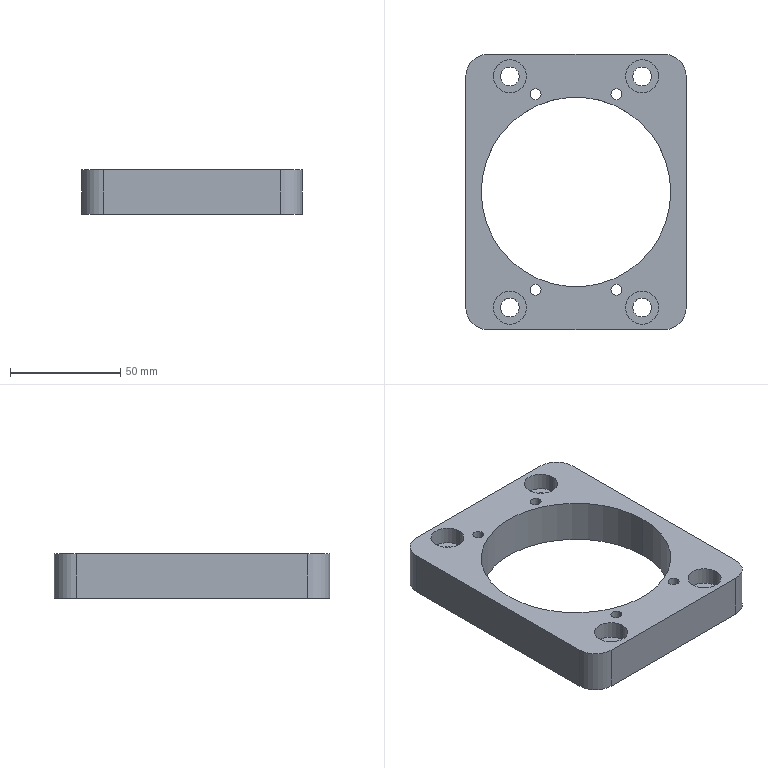Part | SolidWorks | features HoleWzd 2, Extrusion 1, Fillet 1, ICE 1, MirrorPattern 1 | 1 solid | 40 faces | box 100 x 125 x 20 mm | volume 122158 mm3 | cylinder 30 | plane 10 | commonest cylinder face diameters 5 x8 8.5 x8 15 x8 20 x4 86 x2
STEP:
#1=CARTESIAN_POINT('',(-20.869,-44.346,0.));
#2=VERTEX_POINT('',#1);
#3=CARTESIAN_POINT('',(-15.869,-44.346,0.));
#4=VERTEX_POINT('',#3);
#5=CARTESIAN_POINT('',(-18.369,-44.346,0.));
#6=DIRECTION('',(0.,0.,1.));
#7=DIRECTION('',(1.,0.,0.));
#8=AXIS2_PLACEMENT_3D('',#5,#6,#7);
#9=CIRCLE('',#8,2.5);
#10=EDGE_CURVE('',#2,#4,#9,.T.);
#11=ORIENTED_EDGE('',*,*,#10,.F.);
#12=CARTESIAN_POINT('',(-20.869,-44.346,20.));
#13=VERTEX_POINT('',#12);
#14=CARTESIAN_POINT('',(-20.869,-44.346,20.));
#15=DIRECTION('',(0.,0.,1.));
#16=VECTOR('',#15,1000.);
#17=LINE('',#14,#16);
#18=EDGE_CURVE('',#2,#13,#17,.T.);
#19=ORIENTED_EDGE('',*,*,#18,.T.);
#20=CARTESIAN_POINT('',(-15.869,-44.346,20.));
#21=VERTEX_POINT('',#20);
#22=CARTESIAN_POINT('',(-18.369,-44.346,20.));
#23=DIRECTION('',(0.,0.,1.));
#24=DIRECTION('',(1.,0.,0.));
#25=AXIS2_PLACEMENT_3D('',#22,#23,#24);
#26=CIRCLE('',#25,2.5);
#27=EDGE_CURVE('',#13,#21,#26,.T.);
#28=ORIENTED_EDGE('',*,*,#27,.T.);
#29=CARTESIAN_POINT('',(-15.869,-44.346,20.));
#30=DIRECTION('',(0.,0.,1.));
#31=VECTOR('',#30,1000.);
#32=LINE('',#29,#31);
#33=EDGE_CURVE('',#4,#21,#32,.T.);
#34=ORIENTED_EDGE('',*,*,#33,.F.);
#35=EDGE_LOOP('',(#11,#19,#28,#34));
#36=FACE_OUTER_BOUND('',#35,.T.);
#37=CARTESIAN_POINT('',(-18.369,-44.346,20.));
#38=DIRECTION('',(0.,0.,1.));
#39=DIRECTION('',(1.,0.,0.));
#40=AXIS2_PLACEMENT_3D('',#37,#38,#39);
#41=CYLINDRICAL_SURFACE('',#40,2.5);
#42=ADVANCED_FACE('',(#36),#41,.F.);
#43=CARTESIAN_POINT('',(15.869,-44.346,0.));
#44=VERTEX_POINT('',#43);
#45=CARTESIAN_POINT('',(20.869,-44.346,0.));
#46=VERTEX_POINT('',#45);
#47=CARTESIAN_POINT('',(18.369,-44.346,0.));
#48=DIRECTION('',(0.,0.,1.));
#49=DIRECTION('',(1.,0.,0.));
#50=AXIS2_PLACEMENT_3D('',#47,#48,#49);
#51=CIRCLE('',#50,2.5);
#52=EDGE_CURVE('',#44,#46,#51,.T.);
#53=ORIENTED_EDGE('',*,*,#52,.F.);
#54=CARTESIAN_POINT('',(15.869,-44.346,20.));
#55=VERTEX_POINT('',#54);
#56=CARTESIAN_POINT('',(15.869,-44.346,20.));
#57=DIRECTION('',(0.,0.,1.));
#58=VECTOR('',#57,1000.);
#59=LINE('',#56,#58);
#60=EDGE_CURVE('',#44,#55,#59,.T.);
#61=ORIENTED_EDGE('',*,*,#60,.T.);
#62=CARTESIAN_POINT('',(20.869,-44.346,20.));
#63=VERTEX_POINT('',#62);
#64=CARTESIAN_POINT('',(18.369,-44.346,20.));
#65=DIRECTION('',(0.,0.,1.));
#66=DIRECTION('',(1.,0.,0.));
#67=AXIS2_PLACEMENT_3D('',#64,#65,#66);
#68=CIRCLE('',#67,2.5);
#69=EDGE_CURVE('',#55,#63,#68,.T.);
#70=ORIENTED_EDGE('',*,*,#69,.T.);
#71=CARTESIAN_POINT('',(20.869,-44.346,20.));
#72=DIRECTION('',(0.,0.,1.));
#73=VECTOR('',#72,1000.);
#74=LINE('',#71,#73);
#75=EDGE_CURVE('',#46,#63,#74,.T.);
#76=ORIENTED_EDGE('',*,*,#75,.F.);
#77=EDGE_LOOP('',(#53,#61,#70,#76));
#78=FACE_OUTER_BOUND('',#77,.T.);
#79=CARTESIAN_POINT('',(18.369,-44.346,20.));
#80=DIRECTION('',(0.,0.,1.));
#81=DIRECTION('',(1.,0.,0.));
#82=AXIS2_PLACEMENT_3D('',#79,#80,#81);
#83=CYLINDRICAL_SURFACE('',#82,2.5);
#84=ADVANCED_FACE('',(#78),#83,.F.);
#85=CARTESIAN_POINT('',(-37.5,52.5,12.));
#86=VERTEX_POINT('',#85);
#87=CARTESIAN_POINT('',(-22.5,52.5,12.));
#88=VERTEX_POINT('',#87);
#89=CARTESIAN_POINT('',(-30.,52.5,12.));
#90=DIRECTION('',(0.,0.,1.));
#91=DIRECTION('',(1.,0.,0.));
#92=AXIS2_PLACEMENT_3D('',#89,#90,#91);
#93=CIRCLE('',#92,7.5);
#94=EDGE_CURVE('',#86,#88,#93,.T.);
#95=ORIENTED_EDGE('',*,*,#94,.F.);
#96=CARTESIAN_POINT('',(-37.5,52.5,20.));
#97=VERTEX_POINT('',#96);
#98=CARTESIAN_POINT('',(-37.5,52.5,20.));
#99=DIRECTION('',(0.,0.,1.));
#100=VECTOR('',#99,1000.);
#101=LINE('',#98,#100);
#102=EDGE_CURVE('',#86,#97,#101,.T.);
#103=ORIENTED_EDGE('',*,*,#102,.T.);
#104=CARTESIAN_POINT('',(-22.5,52.5,20.));
#105=VERTEX_POINT('',#104);
#106=CARTESIAN_POINT('',(-30.,52.5,20.));
#107=DIRECTION('',(0.,0.,1.));
#108=DIRECTION('',(1.,0.,0.));
#109=AXIS2_PLACEMENT_3D('',#106,#107,#108);
#110=CIRCLE('',#109,7.5);
#111=EDGE_CURVE('',#97,#105,#110,.T.);
#112=ORIENTED_EDGE('',*,*,#111,.T.);
#113=CARTESIAN_POINT('',(-22.5,52.5,20.));
#114=DIRECTION('',(0.,0.,1.));
#115=VECTOR('',#114,1000.);
#116=LINE('',#113,#115);
#117=EDGE_CURVE('',#88,#105,#116,.T.);
#118=ORIENTED_EDGE('',*,*,#117,.F.);
#119=EDGE_LOOP('',(#95,#103,#112,#118));
#120=FACE_OUTER_BOUND('',#119,.T.);
#121=CARTESIAN_POINT('',(-30.,52.5,20.));
#122=DIRECTION('',(0.,0.,1.));
#123=DIRECTION('',(1.,0.,0.));
#124=AXIS2_PLACEMENT_3D('',#121,#122,#123);
#125=CYLINDRICAL_SURFACE('',#124,7.5);
#126=ADVANCED_FACE('',(#120),#125,.F.);
#127=CARTESIAN_POINT('',(-34.25,52.5,0.));
#128=VERTEX_POINT('',#127);
#129=CARTESIAN_POINT('',(-25.75,52.5,0.));
#130=VERTEX_POINT('',#129);
#131=CARTESIAN_POINT('',(-30.,52.5,0.));
#132=DIRECTION('',(0.,0.,1.));
#133=DIRECTION('',(1.,0.,0.));
#134=AXIS2_PLACEMENT_3D('',#131,#132,#133);
#135=CIRCLE('',#134,4.25);
#136=EDGE_CURVE('',#128,#130,#135,.T.);
#137=ORIENTED_EDGE('',*,*,#136,.F.);
#138=CARTESIAN_POINT('',(-34.25,52.5,12.));
#139=VERTEX_POINT('',#138);
#140=CARTESIAN_POINT('',(-34.25,52.5,20.));
#141=DIRECTION('',(0.,0.,1.));
#142=VECTOR('',#141,1000.);
#143=LINE('',#140,#142);
#144=EDGE_CURVE('',#128,#139,#143,.T.);
#145=ORIENTED_EDGE('',*,*,#144,.T.);
#146=CARTESIAN_POINT('',(-25.75,52.5,12.));
#147=VERTEX_POINT('',#146);
#148=CARTESIAN_POINT('',(-30.,52.5,12.));
#149=DIRECTION('',(0.,0.,1.));
#150=DIRECTION('',(1.,0.,0.));
#151=AXIS2_PLACEMENT_3D('',#148,#149,#150);
#152=CIRCLE('',#151,4.25);
#153=EDGE_CURVE('',#139,#147,#152,.T.);
#154=ORIENTED_EDGE('',*,*,#153,.T.);
#155=CARTESIAN_POINT('',(-25.75,52.5,20.));
#156=DIRECTION('',(0.,0.,1.));
#157=VECTOR('',#156,1000.);
#158=LINE('',#155,#157);
#159=EDGE_CURVE('',#130,#147,#158,.T.);
#160=ORIENTED_EDGE('',*,*,#159,.F.);
#161=EDGE_LOOP('',(#137,#145,#154,#160));
#162=FACE_OUTER_BOUND('',#161,.T.);
#163=CARTESIAN_POINT('',(-30.,52.5,20.));
#164=DIRECTION('',(0.,0.,1.));
#165=DIRECTION('',(1.,0.,0.));
#166=AXIS2_PLACEMENT_3D('',#163,#164,#165);
#167=CYLINDRICAL_SURFACE('',#166,4.25);
#168=ADVANCED_FACE('',(#162),#167,.F.);
#169=CARTESIAN_POINT('',(22.5,52.5,12.));
#170=VERTEX_POINT('',#169);
#171=CARTESIAN_POINT('',(37.5,52.5,12.));
#172=VERTEX_POINT('',#171);
#173=CARTESIAN_POINT('',(30.,52.5,12.));
#174=DIRECTION('',(0.,0.,1.));
#175=DIRECTION('',(1.,0.,0.));
#176=AXIS2_PLACEMENT_3D('',#173,#174,#175);
#177=CIRCLE('',#176,7.5);
#178=EDGE_CURVE('',#170,#172,#177,.T.);
#179=ORIENTED_EDGE('',*,*,#178,.F.);
#180=CARTESIAN_POINT('',(22.5,52.5,20.));
#181=VERTEX_POINT('',#180);
#182=CARTESIAN_POINT('',(22.5,52.5,20.));
#183=DIRECTION('',(0.,0.,1.));
#184=VECTOR('',#183,1000.);
#185=LINE('',#182,#184);
#186=EDGE_CURVE('',#170,#181,#185,.T.);
#187=ORIENTED_EDGE('',*,*,#186,.T.);
#188=CARTESIAN_POINT('',(37.5,52.5,20.));
#189=VERTEX_POINT('',#188);
#190=CARTESIAN_POINT('',(30.,52.5,20.));
#191=DIRECTION('',(0.,0.,1.));
#192=DIRECTION('',(1.,0.,0.));
#193=AXIS2_PLACEMENT_3D('',#190,#191,#192);
#194=CIRCLE('',#193,7.5);
#195=EDGE_CURVE('',#181,#189,#194,.T.);
#196=ORIENTED_EDGE('',*,*,#195,.T.);
#197=CARTESIAN_POINT('',(37.5,52.5,20.));
#198=DIRECTION('',(0.,0.,1.));
#199=VECTOR('',#198,1000.);
#200=LINE('',#197,#199);
#201=EDGE_CURVE('',#172,#189,#200,.T.);
#202=ORIENTED_EDGE('',*,*,#201,.F.);
#203=EDGE_LOOP('',(#179,#187,#196,#202));
#204=FACE_OUTER_BOUND('',#203,.T.);
#205=CARTESIAN_POINT('',(30.,52.5,20.));
#206=DIRECTION('',(0.,0.,1.));
#207=DIRECTION('',(1.,0.,0.));
#208=AXIS2_PLACEMENT_3D('',#205,#206,#207);
#209=CYLINDRICAL_SURFACE('',#208,7.5);
#210=ADVANCED_FACE('',(#204),#209,.F.);
#211=CARTESIAN_POINT('',(25.75,52.5,0.));
#212=VERTEX_POINT('',#211);
#213=CARTESIAN_POINT('',(34.25,52.5,0.));
#214=VERTEX_POINT('',#213);
#215=CARTESIAN_POINT('',(30.,52.5,0.));
#216=DIRECTION('',(0.,0.,1.));
#217=DIRECTION('',(1.,0.,0.));
#218=AXIS2_PLACEMENT_3D('',#215,#216,#217);
#219=CIRCLE('',#218,4.25);
#220=EDGE_CURVE('',#212,#214,#219,.T.);
#221=ORIENTED_EDGE('',*,*,#220,.F.);
#222=CARTESIAN_POINT('',(25.75,52.5,12.));
#223=VERTEX_POINT('',#222);
#224=CARTESIAN_POINT('',(25.75,52.5,20.));
#225=DIRECTION('',(0.,0.,1.));
#226=VECTOR('',#225,1000.);
#227=LINE('',#224,#226);
#228=EDGE_CURVE('',#212,#223,#227,.T.);
#229=ORIENTED_EDGE('',*,*,#228,.T.);
#230=CARTESIAN_POINT('',(34.25,52.5,12.));
#231=VERTEX_POINT('',#230);
#232=CARTESIAN_POINT('',(30.,52.5,12.));
#233=DIRECTION('',(0.,0.,1.));
#234=DIRECTION('',(1.,0.,0.));
#235=AXIS2_PLACEMENT_3D('',#232,#233,#234);
#236=CIRCLE('',#235,4.25);
#237=EDGE_CURVE('',#223,#231,#236,.T.);
#238=ORIENTED_EDGE('',*,*,#237,.T.);
#239=CARTESIAN_POINT('',(34.25,52.5,20.));
#240=DIRECTION('',(0.,0.,1.));
#241=VECTOR('',#240,1000.);
#242=LINE('',#239,#241);
#243=EDGE_CURVE('',#214,#231,#242,.T.);
#244=ORIENTED_EDGE('',*,*,#243,.F.);
#245=EDGE_LOOP('',(#221,#229,#238,#244));
#246=FACE_OUTER_BOUND('',#245,.T.);
#247=CARTESIAN_POINT('',(30.,52.5,20.));
#248=DIRECTION('',(0.,0.,1.));
#249=DIRECTION('',(1.,0.,0.));
#250=AXIS2_PLACEMENT_3D('',#247,#248,#249);
#251=CYLINDRICAL_SURFACE('',#250,4.25);
#252=ADVANCED_FACE('',(#246),#251,.F.);
#253=CARTESIAN_POINT('',(-20.869,44.346,0.));
#254=VERTEX_POINT('',#253);
#255=CARTESIAN_POINT('',(-15.869,44.346,0.));
#256=VERTEX_POINT('',#255);
#257=CARTESIAN_POINT('',(-18.369,44.346,0.));
#258=DIRECTION('',(0.,0.,1.));
#259=DIRECTION('',(1.,0.,0.));
#260=AXIS2_PLACEMENT_3D('',#257,#258,#259);
#261=CIRCLE('',#260,2.5);
#262=EDGE_CURVE('',#254,#256,#261,.T.);
#263=ORIENTED_EDGE('',*,*,#262,.F.);
#264=CARTESIAN_POINT('',(-20.869,44.346,20.));
#265=VERTEX_POINT('',#264);
#266=CARTESIAN_POINT('',(-20.869,44.346,20.));
#267=DIRECTION('',(0.,0.,1.));
#268=VECTOR('',#267,1000.);
#269=LINE('',#266,#268);
#270=EDGE_CURVE('',#254,#265,#269,.T.);
#271=ORIENTED_EDGE('',*,*,#270,.T.);
#272=CARTESIAN_POINT('',(-15.869,44.346,20.));
#273=VERTEX_POINT('',#272);
#274=CARTESIAN_POINT('',(-18.369,44.346,20.));
#275=DIRECTION('',(0.,0.,1.));
#276=DIRECTION('',(1.,0.,0.));
#277=AXIS2_PLACEMENT_3D('',#274,#275,#276);
#278=CIRCLE('',#277,2.5);
#279=EDGE_CURVE('',#265,#273,#278,.T.);
#280=ORIENTED_EDGE('',*,*,#279,.T.);
#281=CARTESIAN_POINT('',(-15.869,44.346,20.));
#282=DIRECTION('',(0.,0.,1.));
#283=VECTOR('',#282,1000.);
#284=LINE('',#281,#283);
#285=EDGE_CURVE('',#256,#273,#284,.T.);
#286=ORIENTED_EDGE('',*,*,#285,.F.);
#287=EDGE_LOOP('',(#263,#271,#280,#286));
#288=FACE_OUTER_BOUND('',#287,.T.);
#289=CARTESIAN_POINT('',(-18.369,44.346,20.));
#290=DIRECTION('',(0.,0.,1.));
#291=DIRECTION('',(1.,0.,0.));
#292=AXIS2_PLACEMENT_3D('',#289,#290,#291);
#293=CYLINDRICAL_SURFACE('',#292,2.5);
#294=ADVANCED_FACE('',(#288),#293,.F.);
#295=CARTESIAN_POINT('',(15.869,44.346,0.));
#296=VERTEX_POINT('',#295);
#297=CARTESIAN_POINT('',(20.869,44.346,0.));
#298=VERTEX_POINT('',#297);
#299=CARTESIAN_POINT('',(18.369,44.346,0.));
#300=DIRECTION('',(0.,0.,1.));
#301=DIRECTION('',(1.,0.,0.));
#302=AXIS2_PLACEMENT_3D('',#299,#300,#301);
#303=CIRCLE('',#302,2.5);
#304=EDGE_CURVE('',#296,#298,#303,.T.);
#305=ORIENTED_EDGE('',*,*,#304,.F.);
#306=CARTESIAN_POINT('',(15.869,44.346,20.));
#307=VERTEX_POINT('',#306);
#308=CARTESIAN_POINT('',(15.869,44.346,20.));
#309=DIRECTION('',(0.,0.,1.));
#310=VECTOR('',#309,1000.);
#311=LINE('',#308,#310);
#312=EDGE_CURVE('',#296,#307,#311,.T.);
#313=ORIENTED_EDGE('',*,*,#312,.T.);
#314=CARTESIAN_POINT('',(20.869,44.346,20.));
#315=VERTEX_POINT('',#314);
#316=CARTESIAN_POINT('',(18.369,44.346,20.));
#317=DIRECTION('',(0.,0.,1.));
#318=DIRECTION('',(1.,0.,0.));
#319=AXIS2_PLACEMENT_3D('',#316,#317,#318);
#320=CIRCLE('',#319,2.5);
#321=EDGE_CURVE('',#307,#315,#320,.T.);
#322=ORIENTED_EDGE('',*,*,#321,.T.);
#323=CARTESIAN_POINT('',(20.869,44.346,20.));
#324=DIRECTION('',(0.,0.,1.));
#325=VECTOR('',#324,1000.);
#326=LINE('',#323,#325);
#327=EDGE_CURVE('',#298,#315,#326,.T.);
#328=ORIENTED_EDGE('',*,*,#327,.F.);
#329=EDGE_LOOP('',(#305,#313,#322,#328));
#330=FACE_OUTER_BOUND('',#329,.T.);
#331=CARTESIAN_POINT('',(18.369,44.346,20.));
#332=DIRECTION('',(0.,0.,1.));
#333=DIRECTION('',(1.,0.,0.));
#334=AXIS2_PLACEMENT_3D('',#331,#332,#333);
#335=CYLINDRICAL_SURFACE('',#334,2.5);
#336=ADVANCED_FACE('',(#330),#335,.F.);
#337=CARTESIAN_POINT('',(-43.,0.,0.));
#338=VERTEX_POINT('',#337);
#339=CARTESIAN_POINT('',(43.,0.,0.));
#340=VERTEX_POINT('',#339);
#341=CARTESIAN_POINT('',(0.,0.,0.));
#342=DIRECTION('',(0.,0.,1.));
#343=DIRECTION('',(1.,0.,0.));
#344=AXIS2_PLACEMENT_3D('',#341,#342,#343);
#345=CIRCLE('',#344,43.);
#346=EDGE_CURVE('',#338,#340,#345,.T.);
#347=ORIENTED_EDGE('',*,*,#346,.F.);
#348=CARTESIAN_POINT('',(-43.,0.,20.));
#349=VERTEX_POINT('',#348);
#350=CARTESIAN_POINT('',(-43.,0.,0.));
#351=DIRECTION('',(0.,0.,1.));
#352=VECTOR('',#351,1000.);
#353=LINE('',#350,#352);
#354=EDGE_CURVE('',#338,#349,#353,.T.);
#355=ORIENTED_EDGE('',*,*,#354,.T.);
#356=CARTESIAN_POINT('',(43.,0.,20.));
#357=VERTEX_POINT('',#356);
#358=CARTESIAN_POINT('',(0.,0.,20.));
#359=DIRECTION('',(0.,0.,1.));
#360=DIRECTION('',(1.,0.,0.));
#361=AXIS2_PLACEMENT_3D('',#358,#359,#360);
#362=CIRCLE('',#361,43.);
#363=EDGE_CURVE('',#349,#357,#362,.T.);
#364=ORIENTED_EDGE('',*,*,#363,.T.);
#365=CARTESIAN_POINT('',(43.,0.,0.));
#366=DIRECTION('',(0.,0.,1.));
#367=VECTOR('',#366,1000.);
#368=LINE('',#365,#367);
#369=EDGE_CURVE('',#340,#357,#368,.T.);
#370=ORIENTED_EDGE('',*,*,#369,.F.);
#371=EDGE_LOOP('',(#347,#355,#364,#370));
#372=FACE_OUTER_BOUND('',#371,.T.);
#373=CARTESIAN_POINT('',(0.,0.,0.));
#374=DIRECTION('',(0.,0.,1.));
#375=DIRECTION('',(1.,0.,0.));
#376=AXIS2_PLACEMENT_3D('',#373,#374,#375);
#377=CYLINDRICAL_SURFACE('',#376,43.);
#378=ADVANCED_FACE('',(#372),#377,.F.);
#379=CARTESIAN_POINT('',(-37.5,-52.5,12.));
#380=VERTEX_POINT('',#379);
#381=CARTESIAN_POINT('',(-22.5,-52.5,12.));
#382=VERTEX_POINT('',#381);
#383=CARTESIAN_POINT('',(-30.,-52.5,12.));
#384=DIRECTION('',(0.,0.,1.));
#385=DIRECTION('',(1.,0.,0.));
#386=AXIS2_PLACEMENT_3D('',#383,#384,#385);
#387=CIRCLE('',#386,7.5);
#388=EDGE_CURVE('',#380,#382,#387,.T.);
#389=ORIENTED_EDGE('',*,*,#388,.F.);
#390=CARTESIAN_POINT('',(-37.5,-52.5,20.));
#391=VERTEX_POINT('',#390);
#392=CARTESIAN_POINT('',(-37.5,-52.5,20.));
#393=DIRECTION('',(0.,0.,1.));
#394=VECTOR('',#393,1000.);
#395=LINE('',#392,#394);
#396=EDGE_CURVE('',#380,#391,#395,.T.);
#397=ORIENTED_EDGE('',*,*,#396,.T.);
#398=CARTESIAN_POINT('',(-22.5,-52.5,20.));
#399=VERTEX_POINT('',#398);
#400=CARTESIAN_POINT('',(-30.,-52.5,20.));
#401=DIRECTION('',(0.,0.,1.));
#402=DIRECTION('',(1.,0.,0.));
#403=AXIS2_PLACEMENT_3D('',#400,#401,#402);
#404=CIRCLE('',#403,7.5);
#405=EDGE_CURVE('',#391,#399,#404,.T.);
#406=ORIENTED_EDGE('',*,*,#405,.T.);
#407=CARTESIAN_POINT('',(-22.5,-52.5,20.));
#408=DIRECTION('',(0.,0.,1.));
#409=VECTOR('',#408,1000.);
#410=LINE('',#407,#409);
#411=EDGE_CURVE('',#382,#399,#410,.T.);
#412=ORIENTED_EDGE('',*,*,#411,.F.);
#413=EDGE_LOOP('',(#389,#397,#406,#412));
#414=FACE_OUTER_BOUND('',#413,.T.);
#415=CARTESIAN_POINT('',(-30.,-52.5,20.));
#416=DIRECTION('',(0.,0.,1.));
#417=DIRECTION('',(1.,0.,0.));
#418=AXIS2_PLACEMENT_3D('',#415,#416,#417);
#419=CYLINDRICAL_SURFACE('',#418,7.5);
#420=ADVANCED_FACE('',(#414),#419,.F.);
#421=CARTESIAN_POINT('',(-34.25,-52.5,0.));
#422=VERTEX_POINT('',#421);
#423=CARTESIAN_POINT('',(-25.75,-52.5,0.));
#424=VERTEX_POINT('',#423);
#425=CARTESIAN_POINT('',(-30.,-52.5,0.));
#426=DIRECTION('',(0.,0.,1.));
#427=DIRECTION('',(1.,0.,0.));
#428=AXIS2_PLACEMENT_3D('',#425,#426,#427);
#429=CIRCLE('',#428,4.25);
#430=EDGE_CURVE('',#422,#424,#429,.T.);
#431=ORIENTED_EDGE('',*,*,#430,.F.);
#432=CARTESIAN_POINT('',(-34.25,-52.5,12.));
#433=VERTEX_POINT('',#432);
#434=CARTESIAN_POINT('',(-34.25,-52.5,20.));
#435=DIRECTION('',(0.,0.,1.));
#436=VECTOR('',#435,1000.);
#437=LINE('',#434,#436);
#438=EDGE_CURVE('',#422,#433,#437,.T.);
#439=ORIENTED_EDGE('',*,*,#438,.T.);
#440=CARTESIAN_POINT('',(-25.75,-52.5,12.));
#441=VERTEX_POINT('',#440);
#442=CARTESIAN_POINT('',(-30.,-52.5,12.));
#443=DIRECTION('',(0.,0.,1.));
#444=DIRECTION('',(1.,0.,0.));
#445=AXIS2_PLACEMENT_3D('',#442,#443,#444);
#446=CIRCLE('',#445,4.25);
#447=EDGE_CURVE('',#433,#441,#446,.T.);
#448=ORIENTED_EDGE('',*,*,#447,.T.);
#449=CARTESIAN_POINT('',(-25.75,-52.5,20.));
#450=DIRECTION('',(0.,0.,1.));
#451=VECTOR('',#450,1000.);
#452=LINE('',#449,#451);
#453=EDGE_CURVE('',#424,#441,#452,.T.);
#454=ORIENTED_EDGE('',*,*,#453,.F.);
#455=EDGE_LOOP('',(#431,#439,#448,#454));
#456=FACE_OUTER_BOUND('',#455,.T.);
#457=CARTESIAN_POINT('',(-30.,-52.5,20.));
#458=DIRECTION('',(0.,0.,1.));
#459=DIRECTION('',(1.,0.,0.));
#460=AXIS2_PLACEMENT_3D('',#457,#458,#459);
#461=CYLINDRICAL_SURFACE('',#460,4.25);
#462=ADVANCED_FACE('',(#456),#461,.F.);
#463=CARTESIAN_POINT('',(22.5,-52.5,12.));
#464=VERTEX_POINT('',#463);
#465=CARTESIAN_POINT('',(37.5,-52.5,12.));
#466=VERTEX_POINT('',#465);
#467=CARTESIAN_POINT('',(30.,-52.5,12.));
#468=DIRECTION('',(0.,0.,1.));
#469=DIRECTION('',(1.,0.,0.));
#470=AXIS2_PLACEMENT_3D('',#467,#468,#469);
#471=CIRCLE('',#470,7.5);
#472=EDGE_CURVE('',#464,#466,#471,.T.);
#473=ORIENTED_EDGE('',*,*,#472,.F.);
#474=CARTESIAN_POINT('',(22.5,-52.5,20.));
#475=VERTEX_POINT('',#474);
#476=CARTESIAN_POINT('',(22.5,-52.5,20.));
#477=DIRECTION('',(0.,0.,1.));
#478=VECTOR('',#477,1000.);
#479=LINE('',#476,#478);
#480=EDGE_CURVE('',#464,#475,#479,.T.);
#481=ORIENTED_EDGE('',*,*,#480,.T.);
#482=CARTESIAN_POINT('',(37.5,-52.5,20.));
#483=VERTEX_POINT('',#482);
#484=CARTESIAN_POINT('',(30.,-52.5,20.));
#485=DIRECTION('',(0.,0.,1.));
#486=DIRECTION('',(1.,0.,0.));
#487=AXIS2_PLACEMENT_3D('',#484,#485,#486);
#488=CIRCLE('',#487,7.5);
#489=EDGE_CURVE('',#475,#483,#488,.T.);
#490=ORIENTED_EDGE('',*,*,#489,.T.);
#491=CARTESIAN_POINT('',(37.5,-52.5,20.));
#492=DIRECTION('',(0.,0.,1.));
#493=VECTOR('',#492,1000.);
#494=LINE('',#491,#493);
#495=EDGE_CURVE('',#466,#483,#494,.T.);
#496=ORIENTED_EDGE('',*,*,#495,.F.);
#497=EDGE_LOOP('',(#473,#481,#490,#496));
#498=FACE_OUTER_BOUND('',#497,.T.);
#499=CARTESIAN_POINT('',(30.,-52.5,20.));
#500=DIRECTION('',(0.,0.,1.));
#501=DIRECTION('',(1.,0.,0.));
#502=AXIS2_PLACEMENT_3D('',#499,#500,#501);
#503=CYLINDRICAL_SURFACE('',#502,7.5);
#504=ADVANCED_FACE('',(#498),#503,.F.);
#505=CARTESIAN_POINT('',(25.75,-52.5,0.));
#506=VERTEX_POINT('',#505);
#507=CARTESIAN_POINT('',(34.25,-52.5,0.));
#508=VERTEX_POINT('',#507);
#509=CARTESIAN_POINT('',(30.,-52.5,0.));
#510=DIRECTION('',(0.,0.,1.));
#511=DIRECTION('',(1.,0.,0.));
#512=AXIS2_PLACEMENT_3D('',#509,#510,#511);
#513=CIRCLE('',#512,4.25);
#514=EDGE_CURVE('',#506,#508,#513,.T.);
#515=ORIENTED_EDGE('',*,*,#514,.F.);
#516=CARTESIAN_POINT('',(25.75,-52.5,12.));
#517=VERTEX_POINT('',#516);
#518=CARTESIAN_POINT('',(25.75,-52.5,20.));
#519=DIRECTION('',(0.,0.,1.));
#520=VECTOR('',#519,1000.);
#521=LINE('',#518,#520);
#522=EDGE_CURVE('',#506,#517,#521,.T.);
#523=ORIENTED_EDGE('',*,*,#522,.T.);
#524=CARTESIAN_POINT('',(34.25,-52.5,12.));
#525=VERTEX_POINT('',#524);
#526=CARTESIAN_POINT('',(30.,-52.5,12.));
#527=DIRECTION('',(0.,0.,1.));
#528=DIRECTION('',(1.,0.,0.));
#529=AXIS2_PLACEMENT_3D('',#526,#527,#528);
#530=CIRCLE('',#529,4.25);
#531=EDGE_CURVE('',#517,#525,#530,.T.);
#532=ORIENTED_EDGE('',*,*,#531,.T.);
#533=CARTESIAN_POINT('',(34.25,-52.5,20.));
#534=DIRECTION('',(0.,0.,1.));
#535=VECTOR('',#534,1000.);
#536=LINE('',#533,#535);
#537=EDGE_CURVE('',#508,#525,#536,.T.);
#538=ORIENTED_EDGE('',*,*,#537,.F.);
#539=EDGE_LOOP('',(#515,#523,#532,#538));
#540=FACE_OUTER_BOUND('',#539,.T.);
#541=CARTESIAN_POINT('',(30.,-52.5,20.));
#542=DIRECTION('',(0.,0.,1.));
#543=DIRECTION('',(1.,0.,0.));
#544=AXIS2_PLACEMENT_3D('',#541,#542,#543);
#545=CYLINDRICAL_SURFACE('',#544,4.25);
#546=ADVANCED_FACE('',(#540),#545,.F.);
#547=CARTESIAN_POINT('',(-50.,52.5,0.));
#548=VERTEX_POINT('',#547);
#549=CARTESIAN_POINT('',(-50.,-52.5,0.));
#550=VERTEX_POINT('',#549);
#551=CARTESIAN_POINT('',(-50.,62.5,0.));
#552=DIRECTION('',(0.,-1.,0.));
#553=VECTOR('',#552,1000.);
#554=LINE('',#551,#553);
#555=EDGE_CURVE('',#548,#550,#554,.T.);
#556=ORIENTED_EDGE('',*,*,#555,.T.);
#557=CARTESIAN_POINT('',(-50.,-52.5,20.));
#558=VERTEX_POINT('',#557);
#559=CARTESIAN_POINT('',(-50.,-52.5,20.));
#560=DIRECTION('',(0.,0.,1.));
#561=VECTOR('',#560,1000.);
#562=LINE('',#559,#561);
#563=EDGE_CURVE('',#550,#558,#562,.T.);
#564=ORIENTED_EDGE('',*,*,#563,.T.);
#565=CARTESIAN_POINT('',(-50.,52.5,20.));
#566=VERTEX_POINT('',#565);
#567=CARTESIAN_POINT('',(-50.,62.5,20.));
#568=DIRECTION('',(0.,-1.,0.));
#569=VECTOR('',#568,1000.);
#570=LINE('',#567,#569);
#571=EDGE_CURVE('',#566,#558,#570,.T.);
#572=ORIENTED_EDGE('',*,*,#571,.F.);
#573=CARTESIAN_POINT('',(-50.,52.5,0.));
#574=DIRECTION('',(0.,0.,-1.));
#575=VECTOR('',#574,1000.);
#576=LINE('',#573,#575);
#577=EDGE_CURVE('',#566,#548,#576,.T.);
#578=ORIENTED_EDGE('',*,*,#577,.T.);
#579=EDGE_LOOP('',(#556,#564,#572,#578));
#580=FACE_OUTER_BOUND('',#579,.T.);
#581=CARTESIAN_POINT('',(-50.,62.5,20.));
#582=DIRECTION('',(1.,0.,0.));
#583=DIRECTION('',(0.,1.,0.));
#584=AXIS2_PLACEMENT_3D('',#581,#582,#583);
#585=PLANE('',#584);
#586=ADVANCED_FACE('',(#580),#585,.F.);
#587=CARTESIAN_POINT('',(-40.,-62.5,0.));
#588=VERTEX_POINT('',#587);
#589=CARTESIAN_POINT('',(40.,-62.5,0.));
#590=VERTEX_POINT('',#589);
#591=CARTESIAN_POINT('',(-50.,-62.5,0.));
#592=DIRECTION('',(1.,0.,0.));
#593=VECTOR('',#592,1000.);
#594=LINE('',#591,#593);
#595=EDGE_CURVE('',#588,#590,#594,.T.);
#596=ORIENTED_EDGE('',*,*,#595,.T.);
#597=CARTESIAN_POINT('',(40.,-62.5,20.));
#598=VERTEX_POINT('',#597);
#599=CARTESIAN_POINT('',(40.,-62.5,20.));
#600=DIRECTION('',(0.,0.,1.));
#601=VECTOR('',#600,1000.);
#602=LINE('',#599,#601);
#603=EDGE_CURVE('',#590,#598,#602,.T.);
#604=ORIENTED_EDGE('',*,*,#603,.T.);
#605=CARTESIAN_POINT('',(-40.,-62.5,20.));
#606=VERTEX_POINT('',#605);
#607=CARTESIAN_POINT('',(-50.,-62.5,20.));
#608=DIRECTION('',(1.,0.,0.));
#609=VECTOR('',#608,1000.);
#610=LINE('',#607,#609);
#611=EDGE_CURVE('',#606,#598,#610,.T.);
#612=ORIENTED_EDGE('',*,*,#611,.F.);
#613=CARTESIAN_POINT('',(-40.,-62.5,20.));
#614=DIRECTION('',(0.,0.,-1.));
#615=VECTOR('',#614,1000.);
#616=LINE('',#613,#615);
#617=EDGE_CURVE('',#606,#588,#616,.T.);
#618=ORIENTED_EDGE('',*,*,#617,.T.);
#619=EDGE_LOOP('',(#596,#604,#612,#618));
#620=FACE_OUTER_BOUND('',#619,.T.);
#621=CARTESIAN_POINT('',(-50.,-62.5,20.));
#622=DIRECTION('',(0.,1.,0.));
#623=DIRECTION('',(0.,0.,1.));
#624=AXIS2_PLACEMENT_3D('',#621,#622,#623);
#625=PLANE('',#624);
#626=ADVANCED_FACE('',(#620),#625,.F.);
#627=CARTESIAN_POINT('',(50.,52.5,0.));
#628=VERTEX_POINT('',#627);
#629=CARTESIAN_POINT('',(50.,-52.5,0.));
#630=VERTEX_POINT('',#629);
#631=CARTESIAN_POINT('',(50.,62.5,0.));
#632=DIRECTION('',(0.,-1.,0.));
#633=VECTOR('',#632,1000.);
#634=LINE('',#631,#633);
#635=EDGE_CURVE('',#628,#630,#634,.T.);
#636=ORIENTED_EDGE('',*,*,#635,.F.);
#637=CARTESIAN_POINT('',(50.,52.5,20.));
#638=VERTEX_POINT('',#637);
#639=CARTESIAN_POINT('',(50.,52.5,20.));
#640=DIRECTION('',(0.,0.,1.));
#641=VECTOR('',#640,1000.);
#642=LINE('',#639,#641);
#643=EDGE_CURVE('',#628,#638,#642,.T.);
#644=ORIENTED_EDGE('',*,*,#643,.T.);
#645=CARTESIAN_POINT('',(50.,-52.5,20.));
#646=VERTEX_POINT('',#645);
#647=CARTESIAN_POINT('',(50.,62.5,20.));
#648=DIRECTION('',(0.,-1.,0.));
#649=VECTOR('',#648,1000.);
#650=LINE('',#647,#649);
#651=EDGE_CURVE('',#638,#646,#650,.T.);
#652=ORIENTED_EDGE('',*,*,#651,.T.);
#653=CARTESIAN_POINT('',(50.,-52.5,0.));
#654=DIRECTION('',(0.,0.,-1.));
#655=VECTOR('',#654,1000.);
#656=LINE('',#653,#655);
#657=EDGE_CURVE('',#646,#630,#656,.T.);
#658=ORIENTED_EDGE('',*,*,#657,.T.);
#659=EDGE_LOOP('',(#636,#644,#652,#658));
#660=FACE_OUTER_BOUND('',#659,.T.);
#661=CARTESIAN_POINT('',(50.,62.5,20.));
#662=DIRECTION('',(1.,0.,0.));
#663=DIRECTION('',(0.,1.,0.));
#664=AXIS2_PLACEMENT_3D('',#661,#662,#663);
#665=PLANE('',#664);
#666=ADVANCED_FACE('',(#660),#665,.T.);
#667=CARTESIAN_POINT('',(-40.,62.5,20.));
#668=VERTEX_POINT('',#667);
#669=CARTESIAN_POINT('',(40.,62.5,20.));
#670=VERTEX_POINT('',#669);
#671=CARTESIAN_POINT('',(-50.,62.5,20.));
#672=DIRECTION('',(1.,0.,0.));
#673=VECTOR('',#672,1000.);
#674=LINE('',#671,#673);
#675=EDGE_CURVE('',#668,#670,#674,.T.);
#676=ORIENTED_EDGE('',*,*,#675,.T.);
#677=CARTESIAN_POINT('',(40.,62.5,0.));
#678=VERTEX_POINT('',#677);
#679=CARTESIAN_POINT('',(40.,62.5,20.));
#680=DIRECTION('',(0.,0.,-1.));
#681=VECTOR('',#680,1000.);
#682=LINE('',#679,#681);
#683=EDGE_CURVE('',#670,#678,#682,.T.);
#684=ORIENTED_EDGE('',*,*,#683,.T.);
#685=CARTESIAN_POINT('',(-40.,62.5,0.));
#686=VERTEX_POINT('',#685);
#687=CARTESIAN_POINT('',(-50.,62.5,0.));
#688=DIRECTION('',(1.,0.,0.));
#689=VECTOR('',#688,1000.);
#690=LINE('',#687,#689);
#691=EDGE_CURVE('',#686,#678,#690,.T.);
#692=ORIENTED_EDGE('',*,*,#691,.F.);
#693=CARTESIAN_POINT('',(-40.,62.5,20.));
#694=DIRECTION('',(0.,0.,1.));
#695=VECTOR('',#694,1000.);
#696=LINE('',#693,#695);
#697=EDGE_CURVE('',#686,#668,#696,.T.);
#698=ORIENTED_EDGE('',*,*,#697,.T.);
#699=EDGE_LOOP('',(#676,#684,#692,#698));
#700=FACE_OUTER_BOUND('',#699,.T.);
#701=CARTESIAN_POINT('',(-50.,62.5,20.));
#702=DIRECTION('',(0.,1.,0.));
#703=DIRECTION('',(0.,0.,1.));
#704=AXIS2_PLACEMENT_3D('',#701,#702,#703);
#705=PLANE('',#704);
#706=ADVANCED_FACE('',(#700),#705,.T.);
#707=CARTESIAN_POINT('',(-18.369,-44.346,20.));
#708=DIRECTION('',(0.,0.,1.));
#709=DIRECTION('',(1.,0.,0.));
#710=AXIS2_PLACEMENT_3D('',#707,#708,#709);
#711=CIRCLE('',#710,2.5);
#712=EDGE_CURVE('',#21,#13,#711,.T.);
#713=ORIENTED_EDGE('',*,*,#712,.F.);
#714=ORIENTED_EDGE('',*,*,#27,.F.);
#715=EDGE_LOOP('',(#713,#714));
#716=FACE_BOUND('',#715,.T.);
#717=CARTESIAN_POINT('',(18.369,-44.346,20.));
#718=DIRECTION('',(0.,0.,1.));
#719=DIRECTION('',(1.,0.,0.));
#720=AXIS2_PLACEMENT_3D('',#717,#718,#719);
#721=CIRCLE('',#720,2.5);
#722=EDGE_CURVE('',#63,#55,#721,.T.);
#723=ORIENTED_EDGE('',*,*,#722,.F.);
#724=ORIENTED_EDGE('',*,*,#69,.F.);
#725=EDGE_LOOP('',(#723,#724));
#726=FACE_BOUND('',#725,.T.);
#727=CARTESIAN_POINT('',(-30.,52.5,20.));
#728=DIRECTION('',(0.,0.,1.));
#729=DIRECTION('',(1.,0.,0.));
#730=AXIS2_PLACEMENT_3D('',#727,#728,#729);
#731=CIRCLE('',#730,7.5);
#732=EDGE_CURVE('',#105,#97,#731,.T.);
#733=ORIENTED_EDGE('',*,*,#732,.F.);
#734=ORIENTED_EDGE('',*,*,#111,.F.);
#735=EDGE_LOOP('',(#733,#734));
#736=FACE_BOUND('',#735,.T.);
#737=CARTESIAN_POINT('',(30.,52.5,20.));
#738=DIRECTION('',(0.,0.,1.));
#739=DIRECTION('',(1.,0.,0.));
#740=AXIS2_PLACEMENT_3D('',#737,#738,#739);
#741=CIRCLE('',#740,7.5);
#742=EDGE_CURVE('',#189,#181,#741,.T.);
#743=ORIENTED_EDGE('',*,*,#742,.F.);
#744=ORIENTED_EDGE('',*,*,#195,.F.);
#745=EDGE_LOOP('',(#743,#744));
#746=FACE_BOUND('',#745,.T.);
#747=CARTESIAN_POINT('',(-18.369,44.346,20.));
#748=DIRECTION('',(0.,0.,1.));
#749=DIRECTION('',(1.,0.,0.));
#750=AXIS2_PLACEMENT_3D('',#747,#748,#749);
#751=CIRCLE('',#750,2.5);
#752=EDGE_CURVE('',#273,#265,#751,.T.);
#753=ORIENTED_EDGE('',*,*,#752,.F.);
#754=ORIENTED_EDGE('',*,*,#279,.F.);
#755=EDGE_LOOP('',(#753,#754));
#756=FACE_BOUND('',#755,.T.);
#757=CARTESIAN_POINT('',(18.369,44.346,20.));
#758=DIRECTION('',(0.,0.,1.));
#759=DIRECTION('',(1.,0.,0.));
#760=AXIS2_PLACEMENT_3D('',#757,#758,#759);
#761=CIRCLE('',#760,2.5);
#762=EDGE_CURVE('',#315,#307,#761,.T.);
#763=ORIENTED_EDGE('',*,*,#762,.F.);
#764=ORIENTED_EDGE('',*,*,#321,.F.);
#765=EDGE_LOOP('',(#763,#764));
#766=FACE_BOUND('',#765,.T.);
#767=CARTESIAN_POINT('',(0.,0.,20.));
#768=DIRECTION('',(0.,0.,1.));
#769=DIRECTION('',(1.,0.,0.));
#770=AXIS2_PLACEMENT_3D('',#767,#768,#769);
#771=CIRCLE('',#770,43.);
#772=EDGE_CURVE('',#357,#349,#771,.T.);
#773=ORIENTED_EDGE('',*,*,#772,.F.);
#774=ORIENTED_EDGE('',*,*,#363,.F.);
#775=EDGE_LOOP('',(#773,#774));
#776=FACE_BOUND('',#775,.T.);
#777=CARTESIAN_POINT('',(-30.,-52.5,20.));
#778=DIRECTION('',(0.,0.,1.));
#779=DIRECTION('',(1.,0.,0.));
#780=AXIS2_PLACEMENT_3D('',#777,#778,#779);
#781=CIRCLE('',#780,7.5);
#782=EDGE_CURVE('',#399,#391,#781,.T.);
#783=ORIENTED_EDGE('',*,*,#782,.F.);
#784=ORIENTED_EDGE('',*,*,#405,.F.);
#785=EDGE_LOOP('',(#783,#784));
#786=FACE_BOUND('',#785,.T.);
#787=CARTESIAN_POINT('',(30.,-52.5,20.));
#788=DIRECTION('',(0.,0.,1.));
#789=DIRECTION('',(1.,0.,0.));
#790=AXIS2_PLACEMENT_3D('',#787,#788,#789);
#791=CIRCLE('',#790,7.5);
#792=EDGE_CURVE('',#483,#475,#791,.T.);
#793=ORIENTED_EDGE('',*,*,#792,.F.);
#794=ORIENTED_EDGE('',*,*,#489,.F.);
#795=EDGE_LOOP('',(#793,#794));
#796=FACE_BOUND('',#795,.T.);
#797=ORIENTED_EDGE('',*,*,#651,.F.);
#798=CARTESIAN_POINT('',(40.,52.5,20.));
#799=DIRECTION('',(0.,0.,1.));
#800=DIRECTION('',(1.,0.,0.));
#801=AXIS2_PLACEMENT_3D('',#798,#799,#800);
#802=CIRCLE('',#801,10.);
#803=EDGE_CURVE('',#638,#670,#802,.T.);
#804=ORIENTED_EDGE('',*,*,#803,.T.);
#805=ORIENTED_EDGE('',*,*,#675,.F.);
#806=CARTESIAN_POINT('',(-40.,52.5,20.));
#807=DIRECTION('',(0.,0.,1.));
#808=DIRECTION('',(1.,0.,0.));
#809=AXIS2_PLACEMENT_3D('',#806,#807,#808);
#810=CIRCLE('',#809,10.);
#811=EDGE_CURVE('',#668,#566,#810,.T.);
#812=ORIENTED_EDGE('',*,*,#811,.T.);
#813=ORIENTED_EDGE('',*,*,#571,.T.);
#814=CARTESIAN_POINT('',(-40.,-52.5,20.));
#815=DIRECTION('',(0.,0.,1.));
#816=DIRECTION('',(1.,0.,0.));
#817=AXIS2_PLACEMENT_3D('',#814,#815,#816);
#818=CIRCLE('',#817,10.);
#819=EDGE_CURVE('',#558,#606,#818,.T.);
#820=ORIENTED_EDGE('',*,*,#819,.T.);
#821=ORIENTED_EDGE('',*,*,#611,.T.);
#822=CARTESIAN_POINT('',(40.,-52.5,20.));
#823=DIRECTION('',(0.,0.,1.));
#824=DIRECTION('',(1.,0.,0.));
#825=AXIS2_PLACEMENT_3D('',#822,#823,#824);
#826=CIRCLE('',#825,10.);
#827=EDGE_CURVE('',#598,#646,#826,.T.);
#828=ORIENTED_EDGE('',*,*,#827,.T.);
#829=EDGE_LOOP('',(#797,#804,#805,#812,#813,#820,#821,#828));
#830=FACE_OUTER_BOUND('',#829,.T.);
#831=CARTESIAN_POINT('',(0.,0.,20.));
#832=DIRECTION('',(0.,0.,1.));
#833=DIRECTION('',(1.,0.,0.));
#834=AXIS2_PLACEMENT_3D('',#831,#832,#833);
#835=PLANE('',#834);
#836=ADVANCED_FACE('',(#716,#726,#736,#746,#756,#766,#776,#786,#796,#830),#835,.T.);
#837=CARTESIAN_POINT('',(-18.369,-44.346,0.));
#838=DIRECTION('',(0.,0.,1.));
#839=DIRECTION('',(1.,0.,0.));
#840=AXIS2_PLACEMENT_3D('',#837,#838,#839);
#841=CIRCLE('',#840,2.5);
#842=EDGE_CURVE('',#4,#2,#841,.T.);
#843=ORIENTED_EDGE('',*,*,#842,.T.);
#844=ORIENTED_EDGE('',*,*,#10,.T.);
#845=EDGE_LOOP('',(#843,#844));
#846=FACE_BOUND('',#845,.T.);
#847=CARTESIAN_POINT('',(18.369,-44.346,0.));
#848=DIRECTION('',(0.,0.,1.));
#849=DIRECTION('',(1.,0.,0.));
#850=AXIS2_PLACEMENT_3D('',#847,#848,#849);
#851=CIRCLE('',#850,2.5);
#852=EDGE_CURVE('',#46,#44,#851,.T.);
#853=ORIENTED_EDGE('',*,*,#852,.T.);
#854=ORIENTED_EDGE('',*,*,#52,.T.);
#855=EDGE_LOOP('',(#853,#854));
#856=FACE_BOUND('',#855,.T.);
#857=CARTESIAN_POINT('',(-30.,52.5,0.));
#858=DIRECTION('',(0.,0.,1.));
#859=DIRECTION('',(1.,0.,0.));
#860=AXIS2_PLACEMENT_3D('',#857,#858,#859);
#861=CIRCLE('',#860,4.25);
#862=EDGE_CURVE('',#130,#128,#861,.T.);
#863=ORIENTED_EDGE('',*,*,#862,.T.);
#864=ORIENTED_EDGE('',*,*,#136,.T.);
#865=EDGE_LOOP('',(#863,#864));
#866=FACE_BOUND('',#865,.T.);
#867=CARTESIAN_POINT('',(30.,52.5,0.));
#868=DIRECTION('',(0.,0.,1.));
#869=DIRECTION('',(1.,0.,0.));
#870=AXIS2_PLACEMENT_3D('',#867,#868,#869);
#871=CIRCLE('',#870,4.25);
#872=EDGE_CURVE('',#214,#212,#871,.T.);
#873=ORIENTED_EDGE('',*,*,#872,.T.);
#874=ORIENTED_EDGE('',*,*,#220,.T.);
#875=EDGE_LOOP('',(#873,#874));
#876=FACE_BOUND('',#875,.T.);
#877=CARTESIAN_POINT('',(-18.369,44.346,0.));
#878=DIRECTION('',(0.,0.,1.));
#879=DIRECTION('',(1.,0.,0.));
#880=AXIS2_PLACEMENT_3D('',#877,#878,#879);
#881=CIRCLE('',#880,2.5);
#882=EDGE_CURVE('',#256,#254,#881,.T.);
#883=ORIENTED_EDGE('',*,*,#882,.T.);
#884=ORIENTED_EDGE('',*,*,#262,.T.);
#885=EDGE_LOOP('',(#883,#884));
#886=FACE_BOUND('',#885,.T.);
#887=CARTESIAN_POINT('',(18.369,44.346,0.));
#888=DIRECTION('',(0.,0.,1.));
#889=DIRECTION('',(1.,0.,0.));
#890=AXIS2_PLACEMENT_3D('',#887,#888,#889);
#891=CIRCLE('',#890,2.5);
#892=EDGE_CURVE('',#298,#296,#891,.T.);
#893=ORIENTED_EDGE('',*,*,#892,.T.);
#894=ORIENTED_EDGE('',*,*,#304,.T.);
#895=EDGE_LOOP('',(#893,#894));
#896=FACE_BOUND('',#895,.T.);
#897=CARTESIAN_POINT('',(0.,0.,0.));
#898=DIRECTION('',(0.,0.,1.));
#899=DIRECTION('',(1.,0.,0.));
#900=AXIS2_PLACEMENT_3D('',#897,#898,#899);
#901=CIRCLE('',#900,43.);
#902=EDGE_CURVE('',#340,#338,#901,.T.);
#903=ORIENTED_EDGE('',*,*,#902,.T.);
#904=ORIENTED_EDGE('',*,*,#346,.T.);
#905=EDGE_LOOP('',(#903,#904));
#906=FACE_BOUND('',#905,.T.);
#907=CARTESIAN_POINT('',(-30.,-52.5,0.));
#908=DIRECTION('',(0.,0.,1.));
#909=DIRECTION('',(1.,0.,0.));
#910=AXIS2_PLACEMENT_3D('',#907,#908,#909);
#911=CIRCLE('',#910,4.25);
#912=EDGE_CURVE('',#424,#422,#911,.T.);
#913=ORIENTED_EDGE('',*,*,#912,.T.);
#914=ORIENTED_EDGE('',*,*,#430,.T.);
#915=EDGE_LOOP('',(#913,#914));
#916=FACE_BOUND('',#915,.T.);
#917=CARTESIAN_POINT('',(30.,-52.5,0.));
#918=DIRECTION('',(0.,0.,1.));
#919=DIRECTION('',(1.,0.,0.));
#920=AXIS2_PLACEMENT_3D('',#917,#918,#919);
#921=CIRCLE('',#920,4.25);
#922=EDGE_CURVE('',#508,#506,#921,.T.);
#923=ORIENTED_EDGE('',*,*,#922,.T.);
#924=ORIENTED_EDGE('',*,*,#514,.T.);
#925=EDGE_LOOP('',(#923,#924));
#926=FACE_BOUND('',#925,.T.);
#927=ORIENTED_EDGE('',*,*,#691,.T.);
#928=CARTESIAN_POINT('',(40.,52.5,0.));
#929=DIRECTION('',(0.,0.,-1.));
#930=DIRECTION('',(1.,0.,0.));
#931=AXIS2_PLACEMENT_3D('',#928,#929,#930);
#932=CIRCLE('',#931,10.);
#933=EDGE_CURVE('',#678,#628,#932,.T.);
#934=ORIENTED_EDGE('',*,*,#933,.T.);
#935=ORIENTED_EDGE('',*,*,#635,.T.);
#936=CARTESIAN_POINT('',(40.,-52.5,0.));
#937=DIRECTION('',(0.,0.,-1.));
#938=DIRECTION('',(1.,0.,0.));
#939=AXIS2_PLACEMENT_3D('',#936,#937,#938);
#940=CIRCLE('',#939,10.);
#941=EDGE_CURVE('',#630,#590,#940,.T.);
#942=ORIENTED_EDGE('',*,*,#941,.T.);
#943=ORIENTED_EDGE('',*,*,#595,.F.);
#944=CARTESIAN_POINT('',(-40.,-52.5,0.));
#945=DIRECTION('',(0.,0.,-1.));
#946=DIRECTION('',(1.,0.,0.));
#947=AXIS2_PLACEMENT_3D('',#944,#945,#946);
#948=CIRCLE('',#947,10.);
#949=EDGE_CURVE('',#588,#550,#948,.T.);
#950=ORIENTED_EDGE('',*,*,#949,.T.);
#951=ORIENTED_EDGE('',*,*,#555,.F.);
#952=CARTESIAN_POINT('',(-40.,52.5,0.));
#953=DIRECTION('',(0.,0.,-1.));
#954=DIRECTION('',(1.,0.,0.));
#955=AXIS2_PLACEMENT_3D('',#952,#953,#954);
#956=CIRCLE('',#955,10.);
#957=EDGE_CURVE('',#548,#686,#956,.T.);
#958=ORIENTED_EDGE('',*,*,#957,.T.);
#959=EDGE_LOOP('',(#927,#934,#935,#942,#943,#950,#951,#958));
#960=FACE_OUTER_BOUND('',#959,.T.);
#961=CARTESIAN_POINT('',(0.,0.,0.));
#962=DIRECTION('',(0.,0.,1.));
#963=DIRECTION('',(1.,0.,0.));
#964=AXIS2_PLACEMENT_3D('',#961,#962,#963);
#965=PLANE('',#964);
#966=ADVANCED_FACE('',(#846,#856,#866,#876,#886,#896,#906,#916,#926,#960),#965,.F.);
#967=ORIENTED_EDGE('',*,*,#522,.F.);
#968=ORIENTED_EDGE('',*,*,#922,.F.);
#969=ORIENTED_EDGE('',*,*,#537,.T.);
#970=CARTESIAN_POINT('',(30.,-52.5,12.));
#971=DIRECTION('',(0.,0.,1.));
#972=DIRECTION('',(1.,0.,0.));
#973=AXIS2_PLACEMENT_3D('',#970,#971,#972);
#974=CIRCLE('',#973,4.25);
#975=EDGE_CURVE('',#525,#517,#974,.T.);
#976=ORIENTED_EDGE('',*,*,#975,.T.);
#977=EDGE_LOOP('',(#967,#968,#969,#976));
#978=FACE_OUTER_BOUND('',#977,.T.);
#979=CARTESIAN_POINT('',(30.,-52.5,20.));
#980=DIRECTION('',(0.,0.,1.));
#981=DIRECTION('',(1.,0.,0.));
#982=AXIS2_PLACEMENT_3D('',#979,#980,#981);
#983=CYLINDRICAL_SURFACE('',#982,4.25);
#984=ADVANCED_FACE('',(#978),#983,.F.);
#985=ORIENTED_EDGE('',*,*,#975,.F.);
#986=ORIENTED_EDGE('',*,*,#531,.F.);
#987=EDGE_LOOP('',(#985,#986));
#988=FACE_BOUND('',#987,.T.);
#989=CARTESIAN_POINT('',(30.,-52.5,12.));
#990=DIRECTION('',(0.,0.,1.));
#991=DIRECTION('',(1.,0.,0.));
#992=AXIS2_PLACEMENT_3D('',#989,#990,#991);
#993=CIRCLE('',#992,7.5);
#994=EDGE_CURVE('',#466,#464,#993,.T.);
#995=ORIENTED_EDGE('',*,*,#994,.T.);
#996=ORIENTED_EDGE('',*,*,#472,.T.);
#997=EDGE_LOOP('',(#995,#996));
#998=FACE_OUTER_BOUND('',#997,.T.);
#999=CARTESIAN_POINT('',(34.25,-52.5,12.));
#1000=DIRECTION('',(0.,0.,-1.));
#1001=DIRECTION('',(-1.,0.,0.));
#1002=AXIS2_PLACEMENT_3D('',#999,#1000,#1001);
#1003=PLANE('',#1002);
#1004=ADVANCED_FACE('',(#988,#998),#1003,.F.);
#1005=ORIENTED_EDGE('',*,*,#480,.F.);
#1006=ORIENTED_EDGE('',*,*,#994,.F.);
#1007=ORIENTED_EDGE('',*,*,#495,.T.);
#1008=ORIENTED_EDGE('',*,*,#792,.T.);
#1009=EDGE_LOOP('',(#1005,#1006,#1007,#1008));
#1010=FACE_OUTER_BOUND('',#1009,.T.);
#1011=CARTESIAN_POINT('',(30.,-52.5,20.));
#1012=DIRECTION('',(0.,0.,1.));
#1013=DIRECTION('',(1.,0.,0.));
#1014=AXIS2_PLACEMENT_3D('',#1011,#1012,#1013);
#1015=CYLINDRICAL_SURFACE('',#1014,7.5);
#1016=ADVANCED_FACE('',(#1010),#1015,.F.);
#1017=ORIENTED_EDGE('',*,*,#438,.F.);
#1018=ORIENTED_EDGE('',*,*,#912,.F.);
#1019=ORIENTED_EDGE('',*,*,#453,.T.);
#1020=CARTESIAN_POINT('',(-30.,-52.5,12.));
#1021=DIRECTION('',(0.,0.,1.));
#1022=DIRECTION('',(1.,0.,0.));
#1023=AXIS2_PLACEMENT_3D('',#1020,#1021,#1022);
#1024=CIRCLE('',#1023,4.25);
#1025=EDGE_CURVE('',#441,#433,#1024,.T.);
#1026=ORIENTED_EDGE('',*,*,#1025,.T.);
#1027=EDGE_LOOP('',(#1017,#1018,#1019,#1026));
#1028=FACE_OUTER_BOUND('',#1027,.T.);
#1029=CARTESIAN_POINT('',(-30.,-52.5,20.));
#1030=DIRECTION('',(0.,0.,1.));
#1031=DIRECTION('',(1.,0.,0.));
#1032=AXIS2_PLACEMENT_3D('',#1029,#1030,#1031);
#1033=CYLINDRICAL_SURFACE('',#1032,4.25);
#1034=ADVANCED_FACE('',(#1028),#1033,.F.);
#1035=ORIENTED_EDGE('',*,*,#1025,.F.);
#1036=ORIENTED_EDGE('',*,*,#447,.F.);
#1037=EDGE_LOOP('',(#1035,#1036));
#1038=FACE_BOUND('',#1037,.T.);
#1039=CARTESIAN_POINT('',(-30.,-52.5,12.));
#1040=DIRECTION('',(0.,0.,1.));
#1041=DIRECTION('',(1.,0.,0.));
#1042=AXIS2_PLACEMENT_3D('',#1039,#1040,#1041);
#1043=CIRCLE('',#1042,7.5);
#1044=EDGE_CURVE('',#382,#380,#1043,.T.);
#1045=ORIENTED_EDGE('',*,*,#1044,.T.);
#1046=ORIENTED_EDGE('',*,*,#388,.T.);
#1047=EDGE_LOOP('',(#1045,#1046));
#1048=FACE_OUTER_BOUND('',#1047,.T.);
#1049=CARTESIAN_POINT('',(-25.75,-52.5,12.));
#1050=DIRECTION('',(0.,0.,-1.));
#1051=DIRECTION('',(-1.,0.,0.));
#1052=AXIS2_PLACEMENT_3D('',#1049,#1050,#1051);
#1053=PLANE('',#1052);
#1054=ADVANCED_FACE('',(#1038,#1048),#1053,.F.);
#1055=ORIENTED_EDGE('',*,*,#396,.F.);
#1056=ORIENTED_EDGE('',*,*,#1044,.F.);
#1057=ORIENTED_EDGE('',*,*,#411,.T.);
#1058=ORIENTED_EDGE('',*,*,#782,.T.);
#1059=EDGE_LOOP('',(#1055,#1056,#1057,#1058));
#1060=FACE_OUTER_BOUND('',#1059,.T.);
#1061=CARTESIAN_POINT('',(-30.,-52.5,20.));
#1062=DIRECTION('',(0.,0.,1.));
#1063=DIRECTION('',(1.,0.,0.));
#1064=AXIS2_PLACEMENT_3D('',#1061,#1062,#1063);
#1065=CYLINDRICAL_SURFACE('',#1064,7.5);
#1066=ADVANCED_FACE('',(#1060),#1065,.F.);
#1067=ORIENTED_EDGE('',*,*,#354,.F.);
#1068=ORIENTED_EDGE('',*,*,#902,.F.);
#1069=ORIENTED_EDGE('',*,*,#369,.T.);
#1070=ORIENTED_EDGE('',*,*,#772,.T.);
#1071=EDGE_LOOP('',(#1067,#1068,#1069,#1070));
#1072=FACE_OUTER_BOUND('',#1071,.T.);
#1073=CARTESIAN_POINT('',(0.,0.,0.));
#1074=DIRECTION('',(0.,0.,1.));
#1075=DIRECTION('',(1.,0.,0.));
#1076=AXIS2_PLACEMENT_3D('',#1073,#1074,#1075);
#1077=CYLINDRICAL_SURFACE('',#1076,43.);
#1078=ADVANCED_FACE('',(#1072),#1077,.F.);
#1079=ORIENTED_EDGE('',*,*,#312,.F.);
#1080=ORIENTED_EDGE('',*,*,#892,.F.);
#1081=ORIENTED_EDGE('',*,*,#327,.T.);
#1082=ORIENTED_EDGE('',*,*,#762,.T.);
#1083=EDGE_LOOP('',(#1079,#1080,#1081,#1082));
#1084=FACE_OUTER_BOUND('',#1083,.T.);
#1085=CARTESIAN_POINT('',(18.369,44.346,20.));
#1086=DIRECTION('',(0.,0.,1.));
#1087=DIRECTION('',(1.,0.,0.));
#1088=AXIS2_PLACEMENT_3D('',#1085,#1086,#1087);
#1089=CYLINDRICAL_SURFACE('',#1088,2.5);
#1090=ADVANCED_FACE('',(#1084),#1089,.F.);
#1091=ORIENTED_EDGE('',*,*,#270,.F.);
#1092=ORIENTED_EDGE('',*,*,#882,.F.);
#1093=ORIENTED_EDGE('',*,*,#285,.T.);
#1094=ORIENTED_EDGE('',*,*,#752,.T.);
#1095=EDGE_LOOP('',(#1091,#1092,#1093,#1094));
#1096=FACE_OUTER_BOUND('',#1095,.T.);
#1097=CARTESIAN_POINT('',(-18.369,44.346,20.));
#1098=DIRECTION('',(0.,0.,1.));
#1099=DIRECTION('',(1.,0.,0.));
#1100=AXIS2_PLACEMENT_3D('',#1097,#1098,#1099);
#1101=CYLINDRICAL_SURFACE('',#1100,2.5);
#1102=ADVANCED_FACE('',(#1096),#1101,.F.);
#1103=ORIENTED_EDGE('',*,*,#228,.F.);
#1104=ORIENTED_EDGE('',*,*,#872,.F.);
#1105=ORIENTED_EDGE('',*,*,#243,.T.);
#1106=CARTESIAN_POINT('',(30.,52.5,12.));
#1107=DIRECTION('',(0.,0.,1.));
#1108=DIRECTION('',(1.,0.,0.));
#1109=AXIS2_PLACEMENT_3D('',#1106,#1107,#1108);
#1110=CIRCLE('',#1109,4.25);
#1111=EDGE_CURVE('',#231,#223,#1110,.T.);
#1112=ORIENTED_EDGE('',*,*,#1111,.T.);
#1113=EDGE_LOOP('',(#1103,#1104,#1105,#1112));
#1114=FACE_OUTER_BOUND('',#1113,.T.);
#1115=CARTESIAN_POINT('',(30.,52.5,20.));
#1116=DIRECTION('',(0.,0.,1.));
#1117=DIRECTION('',(1.,0.,0.));
#1118=AXIS2_PLACEMENT_3D('',#1115,#1116,#1117);
#1119=CYLINDRICAL_SURFACE('',#1118,4.25);
#1120=ADVANCED_FACE('',(#1114),#1119,.F.);
#1121=ORIENTED_EDGE('',*,*,#1111,.F.);
#1122=ORIENTED_EDGE('',*,*,#237,.F.);
#1123=EDGE_LOOP('',(#1121,#1122));
#1124=FACE_BOUND('',#1123,.T.);
#1125=CARTESIAN_POINT('',(30.,52.5,12.));
#1126=DIRECTION('',(0.,0.,1.));
#1127=DIRECTION('',(1.,0.,0.));
#1128=AXIS2_PLACEMENT_3D('',#1125,#1126,#1127);
#1129=CIRCLE('',#1128,7.5);
#1130=EDGE_CURVE('',#172,#170,#1129,.T.);
#1131=ORIENTED_EDGE('',*,*,#1130,.T.);
#1132=ORIENTED_EDGE('',*,*,#178,.T.);
#1133=EDGE_LOOP('',(#1131,#1132));
#1134=FACE_OUTER_BOUND('',#1133,.T.);
#1135=CARTESIAN_POINT('',(34.25,52.5,12.));
#1136=DIRECTION('',(0.,0.,-1.));
#1137=DIRECTION('',(-1.,0.,0.));
#1138=AXIS2_PLACEMENT_3D('',#1135,#1136,#1137);
#1139=PLANE('',#1138);
#1140=ADVANCED_FACE('',(#1124,#1134),#1139,.F.);
#1141=ORIENTED_EDGE('',*,*,#186,.F.);
#1142=ORIENTED_EDGE('',*,*,#1130,.F.);
#1143=ORIENTED_EDGE('',*,*,#201,.T.);
#1144=ORIENTED_EDGE('',*,*,#742,.T.);
#1145=EDGE_LOOP('',(#1141,#1142,#1143,#1144));
#1146=FACE_OUTER_BOUND('',#1145,.T.);
#1147=CARTESIAN_POINT('',(30.,52.5,20.));
#1148=DIRECTION('',(0.,0.,1.));
#1149=DIRECTION('',(1.,0.,0.));
#1150=AXIS2_PLACEMENT_3D('',#1147,#1148,#1149);
#1151=CYLINDRICAL_SURFACE('',#1150,7.5);
#1152=ADVANCED_FACE('',(#1146),#1151,.F.);
#1153=ORIENTED_EDGE('',*,*,#144,.F.);
#1154=ORIENTED_EDGE('',*,*,#862,.F.);
#1155=ORIENTED_EDGE('',*,*,#159,.T.);
#1156=CARTESIAN_POINT('',(-30.,52.5,12.));
#1157=DIRECTION('',(0.,0.,1.));
#1158=DIRECTION('',(1.,0.,0.));
#1159=AXIS2_PLACEMENT_3D('',#1156,#1157,#1158);
#1160=CIRCLE('',#1159,4.25);
#1161=EDGE_CURVE('',#147,#139,#1160,.T.);
#1162=ORIENTED_EDGE('',*,*,#1161,.T.);
#1163=EDGE_LOOP('',(#1153,#1154,#1155,#1162));
#1164=FACE_OUTER_BOUND('',#1163,.T.);
#1165=CARTESIAN_POINT('',(-30.,52.5,20.));
#1166=DIRECTION('',(0.,0.,1.));
#1167=DIRECTION('',(1.,0.,0.));
#1168=AXIS2_PLACEMENT_3D('',#1165,#1166,#1167);
#1169=CYLINDRICAL_SURFACE('',#1168,4.25);
#1170=ADVANCED_FACE('',(#1164),#1169,.F.);
#1171=ORIENTED_EDGE('',*,*,#1161,.F.);
#1172=ORIENTED_EDGE('',*,*,#153,.F.);
#1173=EDGE_LOOP('',(#1171,#1172));
#1174=FACE_BOUND('',#1173,.T.);
#1175=CARTESIAN_POINT('',(-30.,52.5,12.));
#1176=DIRECTION('',(0.,0.,1.));
#1177=DIRECTION('',(1.,0.,0.));
#1178=AXIS2_PLACEMENT_3D('',#1175,#1176,#1177);
#1179=CIRCLE('',#1178,7.5);
#1180=EDGE_CURVE('',#88,#86,#1179,.T.);
#1181=ORIENTED_EDGE('',*,*,#1180,.T.);
#1182=ORIENTED_EDGE('',*,*,#94,.T.);
#1183=EDGE_LOOP('',(#1181,#1182));
#1184=FACE_OUTER_BOUND('',#1183,.T.);
#1185=CARTESIAN_POINT('',(-25.75,52.5,12.));
#1186=DIRECTION('',(0.,0.,-1.));
#1187=DIRECTION('',(-1.,0.,0.));
#1188=AXIS2_PLACEMENT_3D('',#1185,#1186,#1187);
#1189=PLANE('',#1188);
#1190=ADVANCED_FACE('',(#1174,#1184),#1189,.F.);
#1191=ORIENTED_EDGE('',*,*,#102,.F.);
#1192=ORIENTED_EDGE('',*,*,#1180,.F.);
#1193=ORIENTED_EDGE('',*,*,#117,.T.);
#1194=ORIENTED_EDGE('',*,*,#732,.T.);
#1195=EDGE_LOOP('',(#1191,#1192,#1193,#1194));
#1196=FACE_OUTER_BOUND('',#1195,.T.);
#1197=CARTESIAN_POINT('',(-30.,52.5,20.));
#1198=DIRECTION('',(0.,0.,1.));
#1199=DIRECTION('',(1.,0.,0.));
#1200=AXIS2_PLACEMENT_3D('',#1197,#1198,#1199);
#1201=CYLINDRICAL_SURFACE('',#1200,7.5);
#1202=ADVANCED_FACE('',(#1196),#1201,.F.);
#1203=ORIENTED_EDGE('',*,*,#60,.F.);
#1204=ORIENTED_EDGE('',*,*,#852,.F.);
#1205=ORIENTED_EDGE('',*,*,#75,.T.);
#1206=ORIENTED_EDGE('',*,*,#722,.T.);
#1207=EDGE_LOOP('',(#1203,#1204,#1205,#1206));
#1208=FACE_OUTER_BOUND('',#1207,.T.);
#1209=CARTESIAN_POINT('',(18.369,-44.346,20.));
#1210=DIRECTION('',(0.,0.,1.));
#1211=DIRECTION('',(1.,0.,0.));
#1212=AXIS2_PLACEMENT_3D('',#1209,#1210,#1211);
#1213=CYLINDRICAL_SURFACE('',#1212,2.5);
#1214=ADVANCED_FACE('',(#1208),#1213,.F.);
#1215=ORIENTED_EDGE('',*,*,#18,.F.);
#1216=ORIENTED_EDGE('',*,*,#842,.F.);
#1217=ORIENTED_EDGE('',*,*,#33,.T.);
#1218=ORIENTED_EDGE('',*,*,#712,.T.);
#1219=EDGE_LOOP('',(#1215,#1216,#1217,#1218));
#1220=FACE_OUTER_BOUND('',#1219,.T.);
#1221=CARTESIAN_POINT('',(-18.369,-44.346,20.));
#1222=DIRECTION('',(0.,0.,1.));
#1223=DIRECTION('',(1.,0.,0.));
#1224=AXIS2_PLACEMENT_3D('',#1221,#1222,#1223);
#1225=CYLINDRICAL_SURFACE('',#1224,2.5);
#1226=ADVANCED_FACE('',(#1220),#1225,.F.);
#1227=ORIENTED_EDGE('',*,*,#803,.F.);
#1228=ORIENTED_EDGE('',*,*,#643,.F.);
#1229=ORIENTED_EDGE('',*,*,#933,.F.);
#1230=ORIENTED_EDGE('',*,*,#683,.F.);
#1231=EDGE_LOOP('',(#1227,#1228,#1229,#1230));
#1232=FACE_OUTER_BOUND('',#1231,.T.);
#1233=CARTESIAN_POINT('',(40.,52.5,20.));
#1234=DIRECTION('',(0.,0.,-1.));
#1235=DIRECTION('',(-1.,0.,0.));
#1236=AXIS2_PLACEMENT_3D('',#1233,#1234,#1235);
#1237=CYLINDRICAL_SURFACE('',#1236,10.);
#1238=ADVANCED_FACE('',(#1232),#1237,.T.);
#1239=ORIENTED_EDGE('',*,*,#827,.F.);
#1240=ORIENTED_EDGE('',*,*,#603,.F.);
#1241=ORIENTED_EDGE('',*,*,#941,.F.);
#1242=ORIENTED_EDGE('',*,*,#657,.F.);
#1243=EDGE_LOOP('',(#1239,#1240,#1241,#1242));
#1244=FACE_OUTER_BOUND('',#1243,.T.);
#1245=CARTESIAN_POINT('',(40.,-52.5,20.));
#1246=DIRECTION('',(0.,0.,1.));
#1247=DIRECTION('',(1.,0.,0.));
#1248=AXIS2_PLACEMENT_3D('',#1245,#1246,#1247);
#1249=CYLINDRICAL_SURFACE('',#1248,10.);
#1250=ADVANCED_FACE('',(#1244),#1249,.T.);
#1251=ORIENTED_EDGE('',*,*,#819,.F.);
#1252=ORIENTED_EDGE('',*,*,#563,.F.);
#1253=ORIENTED_EDGE('',*,*,#949,.F.);
#1254=ORIENTED_EDGE('',*,*,#617,.F.);
#1255=EDGE_LOOP('',(#1251,#1252,#1253,#1254));
#1256=FACE_OUTER_BOUND('',#1255,.T.);
#1257=CARTESIAN_POINT('',(-40.,-52.5,20.));
#1258=DIRECTION('',(0.,0.,-1.));
#1259=DIRECTION('',(-1.,0.,0.));
#1260=AXIS2_PLACEMENT_3D('',#1257,#1258,#1259);
#1261=CYLINDRICAL_SURFACE('',#1260,10.);
#1262=ADVANCED_FACE('',(#1256),#1261,.T.);
#1263=ORIENTED_EDGE('',*,*,#811,.F.);
#1264=ORIENTED_EDGE('',*,*,#697,.F.);
#1265=ORIENTED_EDGE('',*,*,#957,.F.);
#1266=ORIENTED_EDGE('',*,*,#577,.F.);
#1267=EDGE_LOOP('',(#1263,#1264,#1265,#1266));
#1268=FACE_OUTER_BOUND('',#1267,.T.);
#1269=CARTESIAN_POINT('',(-40.,52.5,20.));
#1270=DIRECTION('',(0.,0.,1.));
#1271=DIRECTION('',(1.,0.,0.));
#1272=AXIS2_PLACEMENT_3D('',#1269,#1270,#1271);
#1273=CYLINDRICAL_SURFACE('',#1272,10.);
#1274=ADVANCED_FACE('',(#1268),#1273,.T.);
#1275=CLOSED_SHELL('',(#42,#84,#126,#168,#210,#252,#294,#336,#378,#420,#462,#504,#546,#586,#626,#666,#706,#836,#966,#984,#1004,#1016,#1034,#1054,#1066,#1078,#1090,#1102,#1120,#1140,#1152,#1170,#1190,#1202,#1214,#1226,#1238,#1250,#1262,#1274));
#1276=MANIFOLD_SOLID_BREP('',#1275);
#1277=CARTESIAN_POINT('',(0.,0.,0.));
#1278=DIRECTION('',(0.,0.,1.));
#1279=DIRECTION('',(1.,0.,0.));
#1280=AXIS2_PLACEMENT_3D('',#1277,#1278,#1279);
#1281=(LENGTH_UNIT()NAMED_UNIT(*)SI_UNIT(.MILLI.,.METRE.));
#1282=UNCERTAINTY_MEASURE_WITH_UNIT(LENGTH_MEASURE(0.00001),#1281,'','');
#1283=(NAMED_UNIT(*)PLANE_ANGLE_UNIT()SI_UNIT($,.RADIAN.));
#1284=(NAMED_UNIT(*)SI_UNIT($,.STERADIAN.)SOLID_ANGLE_UNIT());
#1285=(GEOMETRIC_REPRESENTATION_CONTEXT(3)GLOBAL_UNCERTAINTY_ASSIGNED_CONTEXT((#1282))GLOBAL_UNIT_ASSIGNED_CONTEXT((#1281,#1283,#1284))REPRESENTATION_CONTEXT('',''));
#1286=ADVANCED_BREP_SHAPE_REPRESENTATION('',(#1276,#1280),#1285);